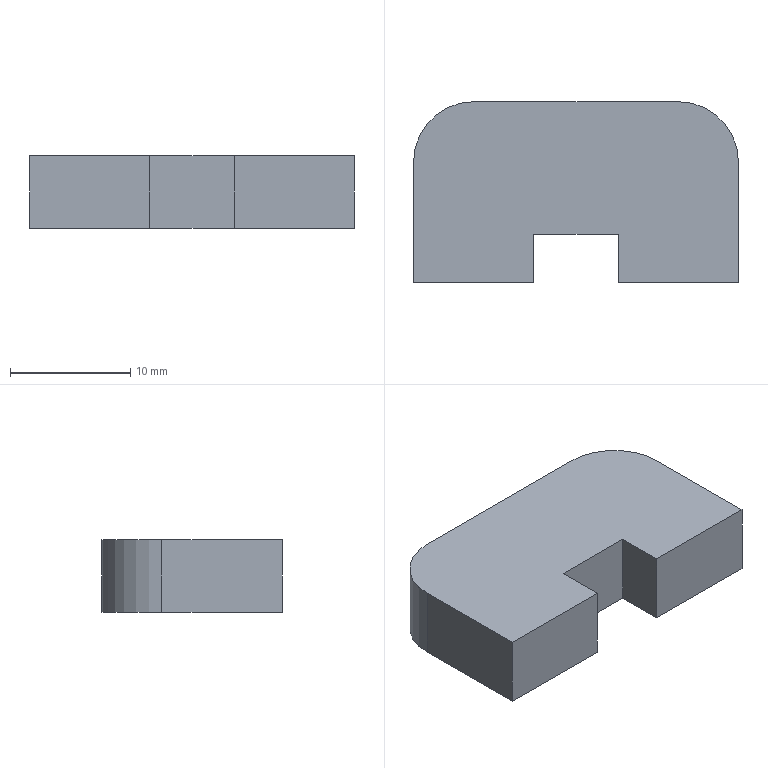Part | SolidWorks | features FlatPattern 1, SMBaseFlange 1, SheetMetal 1 | 1 solid | 12 faces | box 27 x 15 x 6 mm | volume 2198 mm3 | plane 10 | cylinder 2 | commonest cylinder face diameters 10 x2
STEP:
#1=CARTESIAN_POINT('',(-153.47,-549.5,0.));
#2=VERTEX_POINT('',#1);
#3=CARTESIAN_POINT('',(-153.47,-545.5,0.));
#4=VERTEX_POINT('',#3);
#5=CARTESIAN_POINT('',(-153.47,-545.5,0.));
#6=DIRECTION('',(0.,1.,0.));
#7=VECTOR('',#6,1000.);
#8=LINE('',#5,#7);
#9=EDGE_CURVE('',#2,#4,#8,.T.);
#10=ORIENTED_EDGE('',*,*,#9,.F.);
#11=CARTESIAN_POINT('',(-153.47,-549.5,-6.));
#12=VERTEX_POINT('',#11);
#13=CARTESIAN_POINT('',(-153.47,-549.5,-6.));
#14=DIRECTION('',(0.,0.,1.));
#15=VECTOR('',#14,1000.);
#16=LINE('',#13,#15);
#17=EDGE_CURVE('',#12,#2,#16,.T.);
#18=ORIENTED_EDGE('',*,*,#17,.F.);
#19=CARTESIAN_POINT('',(-153.47,-545.5,-6.));
#20=VERTEX_POINT('',#19);
#21=CARTESIAN_POINT('',(-153.47,-545.5,-6.));
#22=DIRECTION('',(0.,1.,0.));
#23=VECTOR('',#22,1000.);
#24=LINE('',#21,#23);
#25=EDGE_CURVE('',#12,#20,#24,.T.);
#26=ORIENTED_EDGE('',*,*,#25,.T.);
#27=CARTESIAN_POINT('',(-153.47,-545.5,-6.));
#28=DIRECTION('',(0.,0.,1.));
#29=VECTOR('',#28,1000.);
#30=LINE('',#27,#29);
#31=EDGE_CURVE('',#20,#4,#30,.T.);
#32=ORIENTED_EDGE('',*,*,#31,.T.);
#33=EDGE_LOOP('',(#10,#18,#26,#32));
#34=FACE_OUTER_BOUND('',#33,.T.);
#35=CARTESIAN_POINT('',(-153.47,-545.5,-6.));
#36=DIRECTION('',(1.,0.,0.));
#37=DIRECTION('',(0.,0.,-1.));
#38=AXIS2_PLACEMENT_3D('',#35,#36,#37);
#39=PLANE('',#38);
#40=ADVANCED_FACE('',(#34),#39,.T.);
#41=CARTESIAN_POINT('',(-163.47,-549.5,0.));
#42=VERTEX_POINT('',#41);
#43=CARTESIAN_POINT('',(-153.47,-549.5,0.));
#44=DIRECTION('',(1.,0.,0.));
#45=VECTOR('',#44,1000.);
#46=LINE('',#43,#45);
#47=EDGE_CURVE('',#42,#2,#46,.T.);
#48=ORIENTED_EDGE('',*,*,#47,.F.);
#49=CARTESIAN_POINT('',(-163.47,-549.5,-6.));
#50=VERTEX_POINT('',#49);
#51=CARTESIAN_POINT('',(-163.47,-549.5,-6.));
#52=DIRECTION('',(0.,0.,1.));
#53=VECTOR('',#52,1000.);
#54=LINE('',#51,#53);
#55=EDGE_CURVE('',#50,#42,#54,.T.);
#56=ORIENTED_EDGE('',*,*,#55,.F.);
#57=CARTESIAN_POINT('',(-153.47,-549.5,-6.));
#58=DIRECTION('',(1.,0.,0.));
#59=VECTOR('',#58,1000.);
#60=LINE('',#57,#59);
#61=EDGE_CURVE('',#50,#12,#60,.T.);
#62=ORIENTED_EDGE('',*,*,#61,.T.);
#63=ORIENTED_EDGE('',*,*,#17,.T.);
#64=EDGE_LOOP('',(#48,#56,#62,#63));
#65=FACE_OUTER_BOUND('',#64,.T.);
#66=CARTESIAN_POINT('',(-153.47,-549.5,-6.));
#67=DIRECTION('',(0.,-1.,0.));
#68=DIRECTION('',(0.,0.,-1.));
#69=AXIS2_PLACEMENT_3D('',#66,#67,#68);
#70=PLANE('',#69);
#71=ADVANCED_FACE('',(#65),#70,.T.);
#72=CARTESIAN_POINT('',(-163.47,-539.5,0.));
#73=VERTEX_POINT('',#72);
#74=CARTESIAN_POINT('',(-163.47,-549.5,0.));
#75=DIRECTION('',(0.,-1.,0.));
#76=VECTOR('',#75,1000.);
#77=LINE('',#74,#76);
#78=EDGE_CURVE('',#73,#42,#77,.T.);
#79=ORIENTED_EDGE('',*,*,#78,.F.);
#80=CARTESIAN_POINT('',(-163.47,-539.5,-6.));
#81=VERTEX_POINT('',#80);
#82=CARTESIAN_POINT('',(-163.47,-539.5,-6.));
#83=DIRECTION('',(0.,0.,1.));
#84=VECTOR('',#83,1000.);
#85=LINE('',#82,#84);
#86=EDGE_CURVE('',#81,#73,#85,.T.);
#87=ORIENTED_EDGE('',*,*,#86,.F.);
#88=CARTESIAN_POINT('',(-163.47,-549.5,-6.));
#89=DIRECTION('',(0.,-1.,0.));
#90=VECTOR('',#89,1000.);
#91=LINE('',#88,#90);
#92=EDGE_CURVE('',#81,#50,#91,.T.);
#93=ORIENTED_EDGE('',*,*,#92,.T.);
#94=ORIENTED_EDGE('',*,*,#55,.T.);
#95=EDGE_LOOP('',(#79,#87,#93,#94));
#96=FACE_OUTER_BOUND('',#95,.T.);
#97=CARTESIAN_POINT('',(-163.47,-549.5,-6.));
#98=DIRECTION('',(-1.,0.,0.));
#99=DIRECTION('',(0.,0.,1.));
#100=AXIS2_PLACEMENT_3D('',#97,#98,#99);
#101=PLANE('',#100);
#102=ADVANCED_FACE('',(#96),#101,.T.);
#103=CARTESIAN_POINT('',(-158.47,-534.5,0.));
#104=VERTEX_POINT('',#103);
#105=CARTESIAN_POINT('',(-158.47,-539.5,0.));
#106=DIRECTION('',(0.,0.,1.));
#107=DIRECTION('',(1.,0.,0.));
#108=AXIS2_PLACEMENT_3D('',#105,#106,#107);
#109=CIRCLE('',#108,5.);
#110=EDGE_CURVE('',#104,#73,#109,.T.);
#111=ORIENTED_EDGE('',*,*,#110,.F.);
#112=CARTESIAN_POINT('',(-158.47,-534.5,-6.));
#113=VERTEX_POINT('',#112);
#114=CARTESIAN_POINT('',(-158.47,-534.5,-6.));
#115=DIRECTION('',(0.,0.,1.));
#116=VECTOR('',#115,1000.);
#117=LINE('',#114,#116);
#118=EDGE_CURVE('',#113,#104,#117,.T.);
#119=ORIENTED_EDGE('',*,*,#118,.F.);
#120=CARTESIAN_POINT('',(-158.47,-539.5,-6.));
#121=DIRECTION('',(0.,0.,1.));
#122=DIRECTION('',(1.,0.,0.));
#123=AXIS2_PLACEMENT_3D('',#120,#121,#122);
#124=CIRCLE('',#123,5.);
#125=EDGE_CURVE('',#113,#81,#124,.T.);
#126=ORIENTED_EDGE('',*,*,#125,.T.);
#127=ORIENTED_EDGE('',*,*,#86,.T.);
#128=EDGE_LOOP('',(#111,#119,#126,#127));
#129=FACE_OUTER_BOUND('',#128,.T.);
#130=CARTESIAN_POINT('',(-158.47,-539.5,-6.));
#131=DIRECTION('',(0.,0.,1.));
#132=DIRECTION('',(1.,0.,0.));
#133=AXIS2_PLACEMENT_3D('',#130,#131,#132);
#134=CYLINDRICAL_SURFACE('',#133,5.);
#135=ADVANCED_FACE('',(#129),#134,.T.);
#136=CARTESIAN_POINT('',(-141.47,-534.5,0.));
#137=VERTEX_POINT('',#136);
#138=CARTESIAN_POINT('',(-141.47,-534.5,0.));
#139=DIRECTION('',(-1.,0.,0.));
#140=VECTOR('',#139,1000.);
#141=LINE('',#138,#140);
#142=EDGE_CURVE('',#137,#104,#141,.T.);
#143=ORIENTED_EDGE('',*,*,#142,.F.);
#144=CARTESIAN_POINT('',(-141.47,-534.5,-6.));
#145=VERTEX_POINT('',#144);
#146=CARTESIAN_POINT('',(-141.47,-534.5,-6.));
#147=DIRECTION('',(0.,0.,1.));
#148=VECTOR('',#147,1000.);
#149=LINE('',#146,#148);
#150=EDGE_CURVE('',#145,#137,#149,.T.);
#151=ORIENTED_EDGE('',*,*,#150,.F.);
#152=CARTESIAN_POINT('',(-141.47,-534.5,-6.));
#153=DIRECTION('',(-1.,0.,0.));
#154=VECTOR('',#153,1000.);
#155=LINE('',#152,#154);
#156=EDGE_CURVE('',#145,#113,#155,.T.);
#157=ORIENTED_EDGE('',*,*,#156,.T.);
#158=ORIENTED_EDGE('',*,*,#118,.T.);
#159=EDGE_LOOP('',(#143,#151,#157,#158));
#160=FACE_OUTER_BOUND('',#159,.T.);
#161=CARTESIAN_POINT('',(-141.47,-534.5,-6.));
#162=DIRECTION('',(0.,1.,0.));
#163=DIRECTION('',(0.,0.,1.));
#164=AXIS2_PLACEMENT_3D('',#161,#162,#163);
#165=PLANE('',#164);
#166=ADVANCED_FACE('',(#160),#165,.T.);
#167=CARTESIAN_POINT('',(-136.47,-539.5,0.));
#168=VERTEX_POINT('',#167);
#169=CARTESIAN_POINT('',(-141.47,-539.5,0.));
#170=DIRECTION('',(0.,0.,1.));
#171=DIRECTION('',(1.,0.,0.));
#172=AXIS2_PLACEMENT_3D('',#169,#170,#171);
#173=CIRCLE('',#172,5.);
#174=EDGE_CURVE('',#168,#137,#173,.T.);
#175=ORIENTED_EDGE('',*,*,#174,.F.);
#176=CARTESIAN_POINT('',(-136.47,-539.5,-6.));
#177=VERTEX_POINT('',#176);
#178=CARTESIAN_POINT('',(-136.47,-539.5,-6.));
#179=DIRECTION('',(0.,0.,1.));
#180=VECTOR('',#179,1000.);
#181=LINE('',#178,#180);
#182=EDGE_CURVE('',#177,#168,#181,.T.);
#183=ORIENTED_EDGE('',*,*,#182,.F.);
#184=CARTESIAN_POINT('',(-141.47,-539.5,-6.));
#185=DIRECTION('',(0.,0.,1.));
#186=DIRECTION('',(1.,0.,0.));
#187=AXIS2_PLACEMENT_3D('',#184,#185,#186);
#188=CIRCLE('',#187,5.);
#189=EDGE_CURVE('',#177,#145,#188,.T.);
#190=ORIENTED_EDGE('',*,*,#189,.T.);
#191=ORIENTED_EDGE('',*,*,#150,.T.);
#192=EDGE_LOOP('',(#175,#183,#190,#191));
#193=FACE_OUTER_BOUND('',#192,.T.);
#194=CARTESIAN_POINT('',(-141.47,-539.5,-6.));
#195=DIRECTION('',(0.,0.,1.));
#196=DIRECTION('',(1.,0.,0.));
#197=AXIS2_PLACEMENT_3D('',#194,#195,#196);
#198=CYLINDRICAL_SURFACE('',#197,5.);
#199=ADVANCED_FACE('',(#193),#198,.T.);
#200=CARTESIAN_POINT('',(-136.47,-549.5,0.));
#201=VERTEX_POINT('',#200);
#202=CARTESIAN_POINT('',(-136.47,-549.5,0.));
#203=DIRECTION('',(0.,1.,0.));
#204=VECTOR('',#203,1000.);
#205=LINE('',#202,#204);
#206=EDGE_CURVE('',#201,#168,#205,.T.);
#207=ORIENTED_EDGE('',*,*,#206,.F.);
#208=CARTESIAN_POINT('',(-136.47,-549.5,-6.));
#209=VERTEX_POINT('',#208);
#210=CARTESIAN_POINT('',(-136.47,-549.5,-6.));
#211=DIRECTION('',(0.,0.,1.));
#212=VECTOR('',#211,1000.);
#213=LINE('',#210,#212);
#214=EDGE_CURVE('',#209,#201,#213,.T.);
#215=ORIENTED_EDGE('',*,*,#214,.F.);
#216=CARTESIAN_POINT('',(-136.47,-549.5,-6.));
#217=DIRECTION('',(0.,1.,0.));
#218=VECTOR('',#217,1000.);
#219=LINE('',#216,#218);
#220=EDGE_CURVE('',#209,#177,#219,.T.);
#221=ORIENTED_EDGE('',*,*,#220,.T.);
#222=ORIENTED_EDGE('',*,*,#182,.T.);
#223=EDGE_LOOP('',(#207,#215,#221,#222));
#224=FACE_OUTER_BOUND('',#223,.T.);
#225=CARTESIAN_POINT('',(-136.47,-549.5,-6.));
#226=DIRECTION('',(1.,0.,0.));
#227=DIRECTION('',(0.,0.,-1.));
#228=AXIS2_PLACEMENT_3D('',#225,#226,#227);
#229=PLANE('',#228);
#230=ADVANCED_FACE('',(#224),#229,.T.);
#231=CARTESIAN_POINT('',(-146.47,-549.5,0.));
#232=VERTEX_POINT('',#231);
#233=CARTESIAN_POINT('',(-146.47,-549.5,0.));
#234=DIRECTION('',(1.,0.,0.));
#235=VECTOR('',#234,1000.);
#236=LINE('',#233,#235);
#237=EDGE_CURVE('',#232,#201,#236,.T.);
#238=ORIENTED_EDGE('',*,*,#237,.F.);
#239=CARTESIAN_POINT('',(-146.47,-549.5,-6.));
#240=VERTEX_POINT('',#239);
#241=CARTESIAN_POINT('',(-146.47,-549.5,-6.));
#242=DIRECTION('',(0.,0.,1.));
#243=VECTOR('',#242,1000.);
#244=LINE('',#241,#243);
#245=EDGE_CURVE('',#240,#232,#244,.T.);
#246=ORIENTED_EDGE('',*,*,#245,.F.);
#247=CARTESIAN_POINT('',(-146.47,-549.5,-6.));
#248=DIRECTION('',(1.,0.,0.));
#249=VECTOR('',#248,1000.);
#250=LINE('',#247,#249);
#251=EDGE_CURVE('',#240,#209,#250,.T.);
#252=ORIENTED_EDGE('',*,*,#251,.T.);
#253=ORIENTED_EDGE('',*,*,#214,.T.);
#254=EDGE_LOOP('',(#238,#246,#252,#253));
#255=FACE_OUTER_BOUND('',#254,.T.);
#256=CARTESIAN_POINT('',(-146.47,-549.5,-6.));
#257=DIRECTION('',(0.,-1.,0.));
#258=DIRECTION('',(0.,0.,-1.));
#259=AXIS2_PLACEMENT_3D('',#256,#257,#258);
#260=PLANE('',#259);
#261=ADVANCED_FACE('',(#255),#260,.T.);
#262=CARTESIAN_POINT('',(-146.47,-545.5,0.));
#263=VERTEX_POINT('',#262);
#264=CARTESIAN_POINT('',(-146.47,-545.5,0.));
#265=DIRECTION('',(0.,-1.,0.));
#266=VECTOR('',#265,1000.);
#267=LINE('',#264,#266);
#268=EDGE_CURVE('',#263,#232,#267,.T.);
#269=ORIENTED_EDGE('',*,*,#268,.F.);
#270=CARTESIAN_POINT('',(-146.47,-545.5,-6.));
#271=VERTEX_POINT('',#270);
#272=CARTESIAN_POINT('',(-146.47,-545.5,-6.));
#273=DIRECTION('',(0.,0.,1.));
#274=VECTOR('',#273,1000.);
#275=LINE('',#272,#274);
#276=EDGE_CURVE('',#271,#263,#275,.T.);
#277=ORIENTED_EDGE('',*,*,#276,.F.);
#278=CARTESIAN_POINT('',(-146.47,-545.5,-6.));
#279=DIRECTION('',(0.,-1.,0.));
#280=VECTOR('',#279,1000.);
#281=LINE('',#278,#280);
#282=EDGE_CURVE('',#271,#240,#281,.T.);
#283=ORIENTED_EDGE('',*,*,#282,.T.);
#284=ORIENTED_EDGE('',*,*,#245,.T.);
#285=EDGE_LOOP('',(#269,#277,#283,#284));
#286=FACE_OUTER_BOUND('',#285,.T.);
#287=CARTESIAN_POINT('',(-146.47,-545.5,-6.));
#288=DIRECTION('',(-1.,0.,0.));
#289=DIRECTION('',(0.,0.,1.));
#290=AXIS2_PLACEMENT_3D('',#287,#288,#289);
#291=PLANE('',#290);
#292=ADVANCED_FACE('',(#286),#291,.T.);
#293=CARTESIAN_POINT('',(-153.47,-545.5,0.));
#294=DIRECTION('',(1.,0.,0.));
#295=VECTOR('',#294,1000.);
#296=LINE('',#293,#295);
#297=EDGE_CURVE('',#4,#263,#296,.T.);
#298=ORIENTED_EDGE('',*,*,#297,.F.);
#299=ORIENTED_EDGE('',*,*,#31,.F.);
#300=CARTESIAN_POINT('',(-153.47,-545.5,-6.));
#301=DIRECTION('',(1.,0.,0.));
#302=VECTOR('',#301,1000.);
#303=LINE('',#300,#302);
#304=EDGE_CURVE('',#20,#271,#303,.T.);
#305=ORIENTED_EDGE('',*,*,#304,.T.);
#306=ORIENTED_EDGE('',*,*,#276,.T.);
#307=EDGE_LOOP('',(#298,#299,#305,#306));
#308=FACE_OUTER_BOUND('',#307,.T.);
#309=CARTESIAN_POINT('',(-153.47,-545.5,-6.));
#310=DIRECTION('',(0.,-1.,0.));
#311=DIRECTION('',(1.,0.,0.));
#312=AXIS2_PLACEMENT_3D('',#309,#310,#311);
#313=PLANE('',#312);
#314=ADVANCED_FACE('',(#308),#313,.T.);
#315=ORIENTED_EDGE('',*,*,#25,.F.);
#316=ORIENTED_EDGE('',*,*,#61,.F.);
#317=ORIENTED_EDGE('',*,*,#92,.F.);
#318=ORIENTED_EDGE('',*,*,#125,.F.);
#319=ORIENTED_EDGE('',*,*,#156,.F.);
#320=ORIENTED_EDGE('',*,*,#189,.F.);
#321=ORIENTED_EDGE('',*,*,#220,.F.);
#322=ORIENTED_EDGE('',*,*,#251,.F.);
#323=ORIENTED_EDGE('',*,*,#282,.F.);
#324=ORIENTED_EDGE('',*,*,#304,.F.);
#325=EDGE_LOOP('',(#315,#316,#317,#318,#319,#320,#321,#322,#323,#324));
#326=FACE_OUTER_BOUND('',#325,.T.);
#327=CARTESIAN_POINT('',(-158.47,-539.5,-6.));
#328=DIRECTION('',(0.,0.,1.));
#329=DIRECTION('',(1.,0.,0.));
#330=AXIS2_PLACEMENT_3D('',#327,#328,#329);
#331=PLANE('',#330);
#332=ADVANCED_FACE('',(#326),#331,.F.);
#333=ORIENTED_EDGE('',*,*,#9,.T.);
#334=ORIENTED_EDGE('',*,*,#297,.T.);
#335=ORIENTED_EDGE('',*,*,#268,.T.);
#336=ORIENTED_EDGE('',*,*,#237,.T.);
#337=ORIENTED_EDGE('',*,*,#206,.T.);
#338=ORIENTED_EDGE('',*,*,#174,.T.);
#339=ORIENTED_EDGE('',*,*,#142,.T.);
#340=ORIENTED_EDGE('',*,*,#110,.T.);
#341=ORIENTED_EDGE('',*,*,#78,.T.);
#342=ORIENTED_EDGE('',*,*,#47,.T.);
#343=EDGE_LOOP('',(#333,#334,#335,#336,#337,#338,#339,#340,#341,#342));
#344=FACE_OUTER_BOUND('',#343,.T.);
#345=CARTESIAN_POINT('',(-158.47,-539.5,0.));
#346=DIRECTION('',(0.,0.,1.));
#347=DIRECTION('',(1.,0.,0.));
#348=AXIS2_PLACEMENT_3D('',#345,#346,#347);
#349=PLANE('',#348);
#350=ADVANCED_FACE('',(#344),#349,.T.);
#351=CLOSED_SHELL('',(#40,#71,#102,#135,#166,#199,#230,#261,#292,#314,#332,#350));
#352=MANIFOLD_SOLID_BREP('',#351);
#353=CARTESIAN_POINT('',(0.,0.,0.));
#354=DIRECTION('',(0.,0.,1.));
#355=DIRECTION('',(1.,0.,0.));
#356=AXIS2_PLACEMENT_3D('',#353,#354,#355);
#357=(LENGTH_UNIT()NAMED_UNIT(*)SI_UNIT(.MILLI.,.METRE.));
#358=UNCERTAINTY_MEASURE_WITH_UNIT(LENGTH_MEASURE(0.00001),#357,'','');
#359=(NAMED_UNIT(*)PLANE_ANGLE_UNIT()SI_UNIT($,.RADIAN.));
#360=(NAMED_UNIT(*)SI_UNIT($,.STERADIAN.)SOLID_ANGLE_UNIT());
#361=(GEOMETRIC_REPRESENTATION_CONTEXT(3)GLOBAL_UNCERTAINTY_ASSIGNED_CONTEXT((#358))GLOBAL_UNIT_ASSIGNED_CONTEXT((#357,#359,#360))REPRESENTATION_CONTEXT('',''));
#362=ADVANCED_BREP_SHAPE_REPRESENTATION('',(#352,#356),#361);